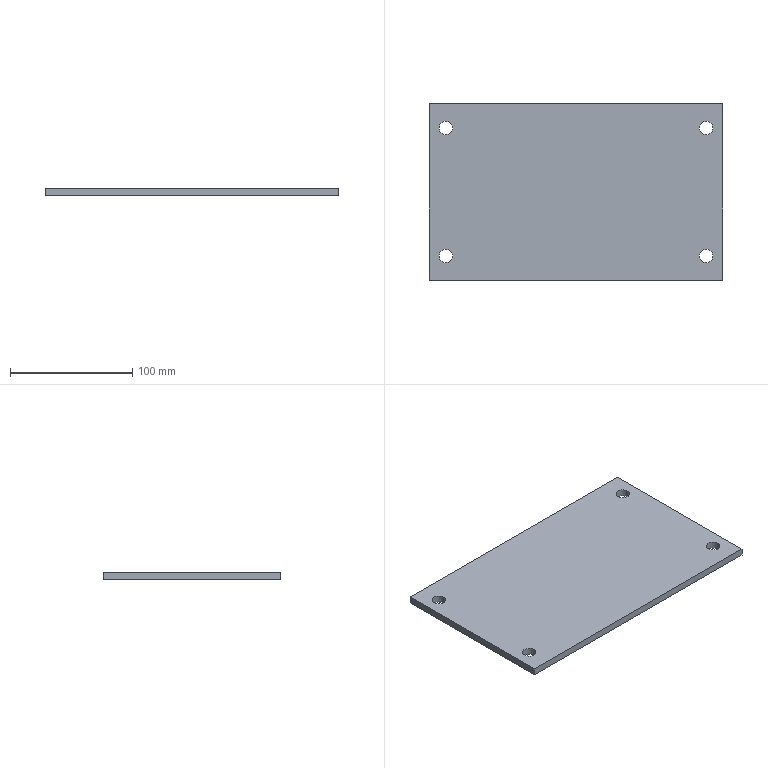Part | SolidWorks | features Extrusion 1, ICE 1, LPattern 1, RefAxis 1 | 1 solid | 14 faces | box 240 x 144 x 6 mm | volume 205079 mm3 | cylinder 8 | plane 6 | commonest cylinder face diameters 11 x8
STEP:
#1=CARTESIAN_POINT('',(100.9,-52.35,0.));
#2=VERTEX_POINT('',#1);
#3=CARTESIAN_POINT('',(111.9,-52.35,0.));
#4=VERTEX_POINT('',#3);
#5=CARTESIAN_POINT('',(106.4,-52.35,0.));
#6=DIRECTION('',(0.,0.,1.));
#7=DIRECTION('',(1.,0.,0.));
#8=AXIS2_PLACEMENT_3D('',#5,#6,#7);
#9=CIRCLE('',#8,5.5);
#10=EDGE_CURVE('',#2,#4,#9,.T.);
#11=ORIENTED_EDGE('',*,*,#10,.F.);
#12=CARTESIAN_POINT('',(100.9,-52.35,6.));
#13=VERTEX_POINT('',#12);
#14=CARTESIAN_POINT('',(100.9,-52.35,0.));
#15=DIRECTION('',(0.,0.,1.));
#16=VECTOR('',#15,1000.);
#17=LINE('',#14,#16);
#18=EDGE_CURVE('',#2,#13,#17,.T.);
#19=ORIENTED_EDGE('',*,*,#18,.T.);
#20=CARTESIAN_POINT('',(111.9,-52.35,6.));
#21=VERTEX_POINT('',#20);
#22=CARTESIAN_POINT('',(106.4,-52.35,6.));
#23=DIRECTION('',(0.,0.,1.));
#24=DIRECTION('',(1.,0.,0.));
#25=AXIS2_PLACEMENT_3D('',#22,#23,#24);
#26=CIRCLE('',#25,5.5);
#27=EDGE_CURVE('',#13,#21,#26,.T.);
#28=ORIENTED_EDGE('',*,*,#27,.T.);
#29=CARTESIAN_POINT('',(111.9,-52.35,0.));
#30=DIRECTION('',(0.,0.,1.));
#31=VECTOR('',#30,1000.);
#32=LINE('',#29,#31);
#33=EDGE_CURVE('',#4,#21,#32,.T.);
#34=ORIENTED_EDGE('',*,*,#33,.F.);
#35=EDGE_LOOP('',(#11,#19,#28,#34));
#36=FACE_OUTER_BOUND('',#35,.T.);
#37=CARTESIAN_POINT('',(106.4,-52.35,0.));
#38=DIRECTION('',(0.,0.,1.));
#39=DIRECTION('',(1.,0.,0.));
#40=AXIS2_PLACEMENT_3D('',#37,#38,#39);
#41=CYLINDRICAL_SURFACE('',#40,5.5);
#42=ADVANCED_FACE('',(#36),#41,.F.);
#43=CARTESIAN_POINT('',(-111.9,-52.35,0.));
#44=VERTEX_POINT('',#43);
#45=CARTESIAN_POINT('',(-100.9,-52.35,0.));
#46=VERTEX_POINT('',#45);
#47=CARTESIAN_POINT('',(-106.4,-52.35,0.));
#48=DIRECTION('',(0.,0.,1.));
#49=DIRECTION('',(1.,0.,0.));
#50=AXIS2_PLACEMENT_3D('',#47,#48,#49);
#51=CIRCLE('',#50,5.5);
#52=EDGE_CURVE('',#44,#46,#51,.T.);
#53=ORIENTED_EDGE('',*,*,#52,.F.);
#54=CARTESIAN_POINT('',(-111.9,-52.35,6.));
#55=VERTEX_POINT('',#54);
#56=CARTESIAN_POINT('',(-111.9,-52.35,0.));
#57=DIRECTION('',(0.,0.,1.));
#58=VECTOR('',#57,1000.);
#59=LINE('',#56,#58);
#60=EDGE_CURVE('',#44,#55,#59,.T.);
#61=ORIENTED_EDGE('',*,*,#60,.T.);
#62=CARTESIAN_POINT('',(-100.9,-52.35,6.));
#63=VERTEX_POINT('',#62);
#64=CARTESIAN_POINT('',(-106.4,-52.35,6.));
#65=DIRECTION('',(0.,0.,1.));
#66=DIRECTION('',(1.,0.,0.));
#67=AXIS2_PLACEMENT_3D('',#64,#65,#66);
#68=CIRCLE('',#67,5.5);
#69=EDGE_CURVE('',#55,#63,#68,.T.);
#70=ORIENTED_EDGE('',*,*,#69,.T.);
#71=CARTESIAN_POINT('',(-100.9,-52.35,0.));
#72=DIRECTION('',(0.,0.,1.));
#73=VECTOR('',#72,1000.);
#74=LINE('',#71,#73);
#75=EDGE_CURVE('',#46,#63,#74,.T.);
#76=ORIENTED_EDGE('',*,*,#75,.F.);
#77=EDGE_LOOP('',(#53,#61,#70,#76));
#78=FACE_OUTER_BOUND('',#77,.T.);
#79=CARTESIAN_POINT('',(-106.4,-52.35,0.));
#80=DIRECTION('',(0.,0.,1.));
#81=DIRECTION('',(1.,0.,0.));
#82=AXIS2_PLACEMENT_3D('',#79,#80,#81);
#83=CYLINDRICAL_SURFACE('',#82,5.5);
#84=ADVANCED_FACE('',(#78),#83,.F.);
#85=CARTESIAN_POINT('',(100.9,52.35,0.));
#86=VERTEX_POINT('',#85);
#87=CARTESIAN_POINT('',(111.9,52.35,0.));
#88=VERTEX_POINT('',#87);
#89=CARTESIAN_POINT('',(106.4,52.35,0.));
#90=DIRECTION('',(0.,0.,1.));
#91=DIRECTION('',(1.,0.,0.));
#92=AXIS2_PLACEMENT_3D('',#89,#90,#91);
#93=CIRCLE('',#92,5.5);
#94=EDGE_CURVE('',#86,#88,#93,.T.);
#95=ORIENTED_EDGE('',*,*,#94,.F.);
#96=CARTESIAN_POINT('',(100.9,52.35,6.));
#97=VERTEX_POINT('',#96);
#98=CARTESIAN_POINT('',(100.9,52.35,0.));
#99=DIRECTION('',(0.,0.,1.));
#100=VECTOR('',#99,1000.);
#101=LINE('',#98,#100);
#102=EDGE_CURVE('',#86,#97,#101,.T.);
#103=ORIENTED_EDGE('',*,*,#102,.T.);
#104=CARTESIAN_POINT('',(111.9,52.35,6.));
#105=VERTEX_POINT('',#104);
#106=CARTESIAN_POINT('',(106.4,52.35,6.));
#107=DIRECTION('',(0.,0.,1.));
#108=DIRECTION('',(1.,0.,0.));
#109=AXIS2_PLACEMENT_3D('',#106,#107,#108);
#110=CIRCLE('',#109,5.5);
#111=EDGE_CURVE('',#97,#105,#110,.T.);
#112=ORIENTED_EDGE('',*,*,#111,.T.);
#113=CARTESIAN_POINT('',(111.9,52.35,0.));
#114=DIRECTION('',(0.,0.,1.));
#115=VECTOR('',#114,1000.);
#116=LINE('',#113,#115);
#117=EDGE_CURVE('',#88,#105,#116,.T.);
#118=ORIENTED_EDGE('',*,*,#117,.F.);
#119=EDGE_LOOP('',(#95,#103,#112,#118));
#120=FACE_OUTER_BOUND('',#119,.T.);
#121=CARTESIAN_POINT('',(106.4,52.35,0.));
#122=DIRECTION('',(0.,0.,1.));
#123=DIRECTION('',(1.,0.,0.));
#124=AXIS2_PLACEMENT_3D('',#121,#122,#123);
#125=CYLINDRICAL_SURFACE('',#124,5.5);
#126=ADVANCED_FACE('',(#120),#125,.F.);
#127=CARTESIAN_POINT('',(-111.9,52.35,0.));
#128=VERTEX_POINT('',#127);
#129=CARTESIAN_POINT('',(-100.9,52.35,0.));
#130=VERTEX_POINT('',#129);
#131=CARTESIAN_POINT('',(-106.4,52.35,0.));
#132=DIRECTION('',(0.,0.,1.));
#133=DIRECTION('',(1.,0.,0.));
#134=AXIS2_PLACEMENT_3D('',#131,#132,#133);
#135=CIRCLE('',#134,5.5);
#136=EDGE_CURVE('',#128,#130,#135,.T.);
#137=ORIENTED_EDGE('',*,*,#136,.F.);
#138=CARTESIAN_POINT('',(-111.9,52.35,6.));
#139=VERTEX_POINT('',#138);
#140=CARTESIAN_POINT('',(-111.9,52.35,0.));
#141=DIRECTION('',(0.,0.,1.));
#142=VECTOR('',#141,1000.);
#143=LINE('',#140,#142);
#144=EDGE_CURVE('',#128,#139,#143,.T.);
#145=ORIENTED_EDGE('',*,*,#144,.T.);
#146=CARTESIAN_POINT('',(-100.9,52.35,6.));
#147=VERTEX_POINT('',#146);
#148=CARTESIAN_POINT('',(-106.4,52.35,6.));
#149=DIRECTION('',(0.,0.,1.));
#150=DIRECTION('',(1.,0.,0.));
#151=AXIS2_PLACEMENT_3D('',#148,#149,#150);
#152=CIRCLE('',#151,5.5);
#153=EDGE_CURVE('',#139,#147,#152,.T.);
#154=ORIENTED_EDGE('',*,*,#153,.T.);
#155=CARTESIAN_POINT('',(-100.9,52.35,0.));
#156=DIRECTION('',(0.,0.,1.));
#157=VECTOR('',#156,1000.);
#158=LINE('',#155,#157);
#159=EDGE_CURVE('',#130,#147,#158,.T.);
#160=ORIENTED_EDGE('',*,*,#159,.F.);
#161=EDGE_LOOP('',(#137,#145,#154,#160));
#162=FACE_OUTER_BOUND('',#161,.T.);
#163=CARTESIAN_POINT('',(-106.4,52.35,0.));
#164=DIRECTION('',(0.,0.,1.));
#165=DIRECTION('',(1.,0.,0.));
#166=AXIS2_PLACEMENT_3D('',#163,#164,#165);
#167=CYLINDRICAL_SURFACE('',#166,5.5);
#168=ADVANCED_FACE('',(#162),#167,.F.);
#169=CARTESIAN_POINT('',(-120.,72.,0.));
#170=VERTEX_POINT('',#169);
#171=CARTESIAN_POINT('',(-120.,-72.,0.));
#172=VERTEX_POINT('',#171);
#173=CARTESIAN_POINT('',(-120.,72.,0.));
#174=DIRECTION('',(0.,-1.,0.));
#175=VECTOR('',#174,1000.);
#176=LINE('',#173,#175);
#177=EDGE_CURVE('',#170,#172,#176,.T.);
#178=ORIENTED_EDGE('',*,*,#177,.T.);
#179=CARTESIAN_POINT('',(-120.,-72.,6.));
#180=VERTEX_POINT('',#179);
#181=CARTESIAN_POINT('',(-120.,-72.,6.));
#182=DIRECTION('',(0.,0.,-1.));
#183=VECTOR('',#182,1000.);
#184=LINE('',#181,#183);
#185=EDGE_CURVE('',#180,#172,#184,.T.);
#186=ORIENTED_EDGE('',*,*,#185,.F.);
#187=CARTESIAN_POINT('',(-120.,72.,6.));
#188=VERTEX_POINT('',#187);
#189=CARTESIAN_POINT('',(-120.,72.,6.));
#190=DIRECTION('',(0.,-1.,0.));
#191=VECTOR('',#190,1000.);
#192=LINE('',#189,#191);
#193=EDGE_CURVE('',#188,#180,#192,.T.);
#194=ORIENTED_EDGE('',*,*,#193,.F.);
#195=CARTESIAN_POINT('',(-120.,72.,6.));
#196=DIRECTION('',(0.,0.,-1.));
#197=VECTOR('',#196,1000.);
#198=LINE('',#195,#197);
#199=EDGE_CURVE('',#188,#170,#198,.T.);
#200=ORIENTED_EDGE('',*,*,#199,.T.);
#201=EDGE_LOOP('',(#178,#186,#194,#200));
#202=FACE_OUTER_BOUND('',#201,.T.);
#203=CARTESIAN_POINT('',(-120.,72.,6.));
#204=DIRECTION('',(1.,0.,0.));
#205=DIRECTION('',(0.,1.,0.));
#206=AXIS2_PLACEMENT_3D('',#203,#204,#205);
#207=PLANE('',#206);
#208=ADVANCED_FACE('',(#202),#207,.F.);
#209=CARTESIAN_POINT('',(120.,-72.,0.));
#210=VERTEX_POINT('',#209);
#211=CARTESIAN_POINT('',(-120.,-72.,0.));
#212=DIRECTION('',(1.,0.,0.));
#213=VECTOR('',#212,1000.);
#214=LINE('',#211,#213);
#215=EDGE_CURVE('',#172,#210,#214,.T.);
#216=ORIENTED_EDGE('',*,*,#215,.T.);
#217=CARTESIAN_POINT('',(120.,-72.,6.));
#218=VERTEX_POINT('',#217);
#219=CARTESIAN_POINT('',(120.,-72.,6.));
#220=DIRECTION('',(0.,0.,-1.));
#221=VECTOR('',#220,1000.);
#222=LINE('',#219,#221);
#223=EDGE_CURVE('',#218,#210,#222,.T.);
#224=ORIENTED_EDGE('',*,*,#223,.F.);
#225=CARTESIAN_POINT('',(-120.,-72.,6.));
#226=DIRECTION('',(1.,0.,0.));
#227=VECTOR('',#226,1000.);
#228=LINE('',#225,#227);
#229=EDGE_CURVE('',#180,#218,#228,.T.);
#230=ORIENTED_EDGE('',*,*,#229,.F.);
#231=ORIENTED_EDGE('',*,*,#185,.T.);
#232=EDGE_LOOP('',(#216,#224,#230,#231));
#233=FACE_OUTER_BOUND('',#232,.T.);
#234=CARTESIAN_POINT('',(-120.,-72.,6.));
#235=DIRECTION('',(0.,1.,0.));
#236=DIRECTION('',(0.,0.,1.));
#237=AXIS2_PLACEMENT_3D('',#234,#235,#236);
#238=PLANE('',#237);
#239=ADVANCED_FACE('',(#233),#238,.F.);
#240=CARTESIAN_POINT('',(120.,72.,0.));
#241=VERTEX_POINT('',#240);
#242=CARTESIAN_POINT('',(120.,72.,0.));
#243=DIRECTION('',(0.,1.,0.));
#244=VECTOR('',#243,1000.);
#245=LINE('',#242,#244);
#246=EDGE_CURVE('',#210,#241,#245,.T.);
#247=ORIENTED_EDGE('',*,*,#246,.T.);
#248=CARTESIAN_POINT('',(120.,72.,6.));
#249=VERTEX_POINT('',#248);
#250=CARTESIAN_POINT('',(120.,72.,6.));
#251=DIRECTION('',(0.,0.,-1.));
#252=VECTOR('',#251,1000.);
#253=LINE('',#250,#252);
#254=EDGE_CURVE('',#249,#241,#253,.T.);
#255=ORIENTED_EDGE('',*,*,#254,.F.);
#256=CARTESIAN_POINT('',(120.,72.,6.));
#257=DIRECTION('',(0.,1.,0.));
#258=VECTOR('',#257,1000.);
#259=LINE('',#256,#258);
#260=EDGE_CURVE('',#218,#249,#259,.T.);
#261=ORIENTED_EDGE('',*,*,#260,.F.);
#262=ORIENTED_EDGE('',*,*,#223,.T.);
#263=EDGE_LOOP('',(#247,#255,#261,#262));
#264=FACE_OUTER_BOUND('',#263,.T.);
#265=CARTESIAN_POINT('',(120.,72.,6.));
#266=DIRECTION('',(-1.,0.,0.));
#267=DIRECTION('',(0.,-1.,0.));
#268=AXIS2_PLACEMENT_3D('',#265,#266,#267);
#269=PLANE('',#268);
#270=ADVANCED_FACE('',(#264),#269,.F.);
#271=CARTESIAN_POINT('',(-120.,72.,0.));
#272=DIRECTION('',(-1.,0.,0.));
#273=VECTOR('',#272,1000.);
#274=LINE('',#271,#273);
#275=EDGE_CURVE('',#241,#170,#274,.T.);
#276=ORIENTED_EDGE('',*,*,#275,.T.);
#277=ORIENTED_EDGE('',*,*,#199,.F.);
#278=CARTESIAN_POINT('',(-120.,72.,6.));
#279=DIRECTION('',(-1.,0.,0.));
#280=VECTOR('',#279,1000.);
#281=LINE('',#278,#280);
#282=EDGE_CURVE('',#249,#188,#281,.T.);
#283=ORIENTED_EDGE('',*,*,#282,.F.);
#284=ORIENTED_EDGE('',*,*,#254,.T.);
#285=EDGE_LOOP('',(#276,#277,#283,#284));
#286=FACE_OUTER_BOUND('',#285,.T.);
#287=CARTESIAN_POINT('',(-120.,72.,6.));
#288=DIRECTION('',(0.,-1.,0.));
#289=DIRECTION('',(0.,0.,-1.));
#290=AXIS2_PLACEMENT_3D('',#287,#288,#289);
#291=PLANE('',#290);
#292=ADVANCED_FACE('',(#286),#291,.F.);
#293=CARTESIAN_POINT('',(106.4,52.35,6.));
#294=DIRECTION('',(0.,0.,1.));
#295=DIRECTION('',(1.,0.,0.));
#296=AXIS2_PLACEMENT_3D('',#293,#294,#295);
#297=CIRCLE('',#296,5.5);
#298=EDGE_CURVE('',#105,#97,#297,.T.);
#299=ORIENTED_EDGE('',*,*,#298,.F.);
#300=ORIENTED_EDGE('',*,*,#111,.F.);
#301=EDGE_LOOP('',(#299,#300));
#302=FACE_BOUND('',#301,.T.);
#303=CARTESIAN_POINT('',(-106.4,52.35,6.));
#304=DIRECTION('',(0.,0.,1.));
#305=DIRECTION('',(1.,0.,0.));
#306=AXIS2_PLACEMENT_3D('',#303,#304,#305);
#307=CIRCLE('',#306,5.5);
#308=EDGE_CURVE('',#147,#139,#307,.T.);
#309=ORIENTED_EDGE('',*,*,#308,.F.);
#310=ORIENTED_EDGE('',*,*,#153,.F.);
#311=EDGE_LOOP('',(#309,#310));
#312=FACE_BOUND('',#311,.T.);
#313=ORIENTED_EDGE('',*,*,#193,.T.);
#314=ORIENTED_EDGE('',*,*,#229,.T.);
#315=ORIENTED_EDGE('',*,*,#260,.T.);
#316=ORIENTED_EDGE('',*,*,#282,.T.);
#317=EDGE_LOOP('',(#313,#314,#315,#316));
#318=FACE_OUTER_BOUND('',#317,.T.);
#319=CARTESIAN_POINT('',(-106.4,-52.35,6.));
#320=DIRECTION('',(0.,0.,1.));
#321=DIRECTION('',(1.,0.,0.));
#322=AXIS2_PLACEMENT_3D('',#319,#320,#321);
#323=CIRCLE('',#322,5.5);
#324=EDGE_CURVE('',#63,#55,#323,.T.);
#325=ORIENTED_EDGE('',*,*,#324,.F.);
#326=ORIENTED_EDGE('',*,*,#69,.F.);
#327=EDGE_LOOP('',(#325,#326));
#328=FACE_BOUND('',#327,.T.);
#329=CARTESIAN_POINT('',(106.4,-52.35,6.));
#330=DIRECTION('',(0.,0.,1.));
#331=DIRECTION('',(1.,0.,0.));
#332=AXIS2_PLACEMENT_3D('',#329,#330,#331);
#333=CIRCLE('',#332,5.5);
#334=EDGE_CURVE('',#21,#13,#333,.T.);
#335=ORIENTED_EDGE('',*,*,#334,.F.);
#336=ORIENTED_EDGE('',*,*,#27,.F.);
#337=EDGE_LOOP('',(#335,#336));
#338=FACE_BOUND('',#337,.T.);
#339=CARTESIAN_POINT('',(0.,0.,6.));
#340=DIRECTION('',(0.,0.,1.));
#341=DIRECTION('',(1.,0.,0.));
#342=AXIS2_PLACEMENT_3D('',#339,#340,#341);
#343=PLANE('',#342);
#344=ADVANCED_FACE('',(#302,#312,#318,#328,#338),#343,.T.);
#345=CARTESIAN_POINT('',(106.4,52.35,0.));
#346=DIRECTION('',(0.,0.,1.));
#347=DIRECTION('',(1.,0.,0.));
#348=AXIS2_PLACEMENT_3D('',#345,#346,#347);
#349=CIRCLE('',#348,5.5);
#350=EDGE_CURVE('',#88,#86,#349,.T.);
#351=ORIENTED_EDGE('',*,*,#350,.T.);
#352=ORIENTED_EDGE('',*,*,#94,.T.);
#353=EDGE_LOOP('',(#351,#352));
#354=FACE_BOUND('',#353,.T.);
#355=CARTESIAN_POINT('',(-106.4,52.35,0.));
#356=DIRECTION('',(0.,0.,1.));
#357=DIRECTION('',(1.,0.,0.));
#358=AXIS2_PLACEMENT_3D('',#355,#356,#357);
#359=CIRCLE('',#358,5.5);
#360=EDGE_CURVE('',#130,#128,#359,.T.);
#361=ORIENTED_EDGE('',*,*,#360,.T.);
#362=ORIENTED_EDGE('',*,*,#136,.T.);
#363=EDGE_LOOP('',(#361,#362));
#364=FACE_BOUND('',#363,.T.);
#365=ORIENTED_EDGE('',*,*,#177,.F.);
#366=ORIENTED_EDGE('',*,*,#275,.F.);
#367=ORIENTED_EDGE('',*,*,#246,.F.);
#368=ORIENTED_EDGE('',*,*,#215,.F.);
#369=EDGE_LOOP('',(#365,#366,#367,#368));
#370=FACE_OUTER_BOUND('',#369,.T.);
#371=CARTESIAN_POINT('',(-106.4,-52.35,0.));
#372=DIRECTION('',(0.,0.,1.));
#373=DIRECTION('',(1.,0.,0.));
#374=AXIS2_PLACEMENT_3D('',#371,#372,#373);
#375=CIRCLE('',#374,5.5);
#376=EDGE_CURVE('',#46,#44,#375,.T.);
#377=ORIENTED_EDGE('',*,*,#376,.T.);
#378=ORIENTED_EDGE('',*,*,#52,.T.);
#379=EDGE_LOOP('',(#377,#378));
#380=FACE_BOUND('',#379,.T.);
#381=CARTESIAN_POINT('',(106.4,-52.35,0.));
#382=DIRECTION('',(0.,0.,1.));
#383=DIRECTION('',(1.,0.,0.));
#384=AXIS2_PLACEMENT_3D('',#381,#382,#383);
#385=CIRCLE('',#384,5.5);
#386=EDGE_CURVE('',#4,#2,#385,.T.);
#387=ORIENTED_EDGE('',*,*,#386,.T.);
#388=ORIENTED_EDGE('',*,*,#10,.T.);
#389=EDGE_LOOP('',(#387,#388));
#390=FACE_BOUND('',#389,.T.);
#391=CARTESIAN_POINT('',(0.,0.,0.));
#392=DIRECTION('',(0.,0.,1.));
#393=DIRECTION('',(1.,0.,0.));
#394=AXIS2_PLACEMENT_3D('',#391,#392,#393);
#395=PLANE('',#394);
#396=ADVANCED_FACE('',(#354,#364,#370,#380,#390),#395,.F.);
#397=ORIENTED_EDGE('',*,*,#144,.F.);
#398=ORIENTED_EDGE('',*,*,#360,.F.);
#399=ORIENTED_EDGE('',*,*,#159,.T.);
#400=ORIENTED_EDGE('',*,*,#308,.T.);
#401=EDGE_LOOP('',(#397,#398,#399,#400));
#402=FACE_OUTER_BOUND('',#401,.T.);
#403=CARTESIAN_POINT('',(-106.4,52.35,0.));
#404=DIRECTION('',(0.,0.,1.));
#405=DIRECTION('',(1.,0.,0.));
#406=AXIS2_PLACEMENT_3D('',#403,#404,#405);
#407=CYLINDRICAL_SURFACE('',#406,5.5);
#408=ADVANCED_FACE('',(#402),#407,.F.);
#409=ORIENTED_EDGE('',*,*,#102,.F.);
#410=ORIENTED_EDGE('',*,*,#350,.F.);
#411=ORIENTED_EDGE('',*,*,#117,.T.);
#412=ORIENTED_EDGE('',*,*,#298,.T.);
#413=EDGE_LOOP('',(#409,#410,#411,#412));
#414=FACE_OUTER_BOUND('',#413,.T.);
#415=CARTESIAN_POINT('',(106.4,52.35,0.));
#416=DIRECTION('',(0.,0.,1.));
#417=DIRECTION('',(1.,0.,0.));
#418=AXIS2_PLACEMENT_3D('',#415,#416,#417);
#419=CYLINDRICAL_SURFACE('',#418,5.5);
#420=ADVANCED_FACE('',(#414),#419,.F.);
#421=ORIENTED_EDGE('',*,*,#60,.F.);
#422=ORIENTED_EDGE('',*,*,#376,.F.);
#423=ORIENTED_EDGE('',*,*,#75,.T.);
#424=ORIENTED_EDGE('',*,*,#324,.T.);
#425=EDGE_LOOP('',(#421,#422,#423,#424));
#426=FACE_OUTER_BOUND('',#425,.T.);
#427=CARTESIAN_POINT('',(-106.4,-52.35,0.));
#428=DIRECTION('',(0.,0.,1.));
#429=DIRECTION('',(1.,0.,0.));
#430=AXIS2_PLACEMENT_3D('',#427,#428,#429);
#431=CYLINDRICAL_SURFACE('',#430,5.5);
#432=ADVANCED_FACE('',(#426),#431,.F.);
#433=ORIENTED_EDGE('',*,*,#18,.F.);
#434=ORIENTED_EDGE('',*,*,#386,.F.);
#435=ORIENTED_EDGE('',*,*,#33,.T.);
#436=ORIENTED_EDGE('',*,*,#334,.T.);
#437=EDGE_LOOP('',(#433,#434,#435,#436));
#438=FACE_OUTER_BOUND('',#437,.T.);
#439=CARTESIAN_POINT('',(106.4,-52.35,0.));
#440=DIRECTION('',(0.,0.,1.));
#441=DIRECTION('',(1.,0.,0.));
#442=AXIS2_PLACEMENT_3D('',#439,#440,#441);
#443=CYLINDRICAL_SURFACE('',#442,5.5);
#444=ADVANCED_FACE('',(#438),#443,.F.);
#445=CLOSED_SHELL('',(#42,#84,#126,#168,#208,#239,#270,#292,#344,#396,#408,#420,#432,#444));
#446=MANIFOLD_SOLID_BREP('',#445);
#447=CARTESIAN_POINT('',(0.,0.,0.));
#448=DIRECTION('',(0.,0.,1.));
#449=DIRECTION('',(1.,0.,0.));
#450=AXIS2_PLACEMENT_3D('',#447,#448,#449);
#451=(LENGTH_UNIT()NAMED_UNIT(*)SI_UNIT(.MILLI.,.METRE.));
#452=UNCERTAINTY_MEASURE_WITH_UNIT(LENGTH_MEASURE(0.00001),#451,'','');
#453=(NAMED_UNIT(*)PLANE_ANGLE_UNIT()SI_UNIT($,.RADIAN.));
#454=(NAMED_UNIT(*)SI_UNIT($,.STERADIAN.)SOLID_ANGLE_UNIT());
#455=(GEOMETRIC_REPRESENTATION_CONTEXT(3)GLOBAL_UNCERTAINTY_ASSIGNED_CONTEXT((#452))GLOBAL_UNIT_ASSIGNED_CONTEXT((#451,#453,#454))REPRESENTATION_CONTEXT('',''));
#456=ADVANCED_BREP_SHAPE_REPRESENTATION('',(#446,#450),#455);